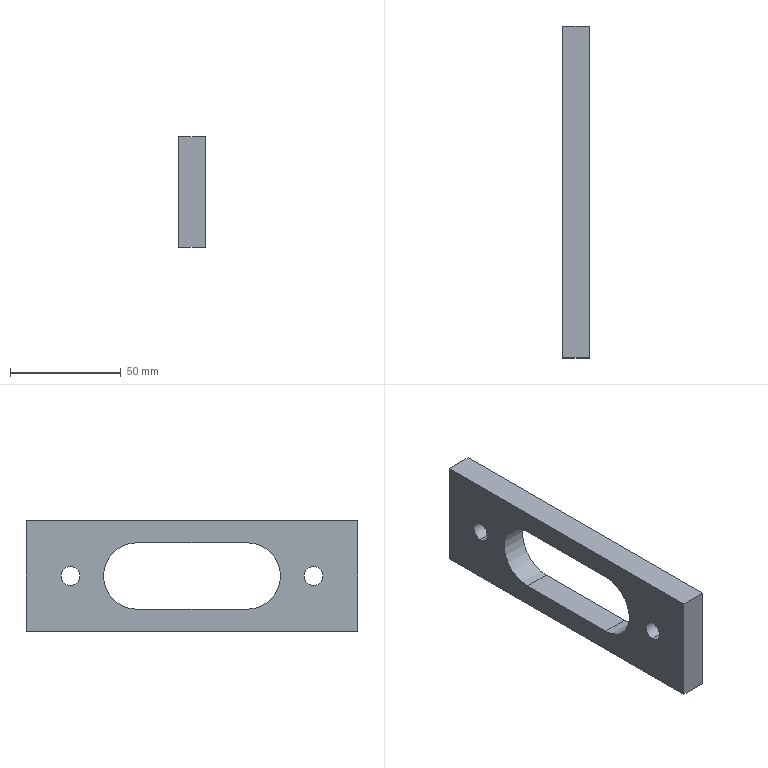Part | SolidWorks | features BaseBody 1 | 1 solid | 14 faces | box 12 x 150 x 50 mm | volume 62156 mm3 | plane 8 | cylinder 6 | commonest cylinder face diameters 8.5 x4 30 x2
STEP:
#1=CARTESIAN_POINT('',(-13.,224.,4.25));
#2=VERTEX_POINT('',#1);
#3=CARTESIAN_POINT('',(-13.,224.,-4.25));
#4=VERTEX_POINT('',#3);
#5=CARTESIAN_POINT('',(-13.,224.,0.));
#6=DIRECTION('',(1.,0.,0.));
#7=DIRECTION('',(0.,0.,-1.));
#8=AXIS2_PLACEMENT_3D('',#5,#6,#7);
#9=CIRCLE('',#8,4.25);
#10=EDGE_CURVE('',#2,#4,#9,.T.);
#11=ORIENTED_EDGE('',*,*,#10,.T.);
#12=CARTESIAN_POINT('',(-25.,224.,-4.25));
#13=VERTEX_POINT('',#12);
#14=CARTESIAN_POINT('',(-25.,224.,-4.25));
#15=DIRECTION('',(-1.,0.,0.));
#16=VECTOR('',#15,1000.);
#17=LINE('',#14,#16);
#18=EDGE_CURVE('',#4,#13,#17,.T.);
#19=ORIENTED_EDGE('',*,*,#18,.T.);
#20=CARTESIAN_POINT('',(-25.,224.,4.25));
#21=VERTEX_POINT('',#20);
#22=CARTESIAN_POINT('',(-25.,224.,0.));
#23=DIRECTION('',(1.,0.,0.));
#24=DIRECTION('',(0.,0.,1.));
#25=AXIS2_PLACEMENT_3D('',#22,#23,#24);
#26=CIRCLE('',#25,4.25);
#27=EDGE_CURVE('',#21,#13,#26,.T.);
#28=ORIENTED_EDGE('',*,*,#27,.F.);
#29=CARTESIAN_POINT('',(-25.,224.,4.25));
#30=DIRECTION('',(-1.,0.,0.));
#31=VECTOR('',#30,1000.);
#32=LINE('',#29,#31);
#33=EDGE_CURVE('',#2,#21,#32,.T.);
#34=ORIENTED_EDGE('',*,*,#33,.F.);
#35=EDGE_LOOP('',(#11,#19,#28,#34));
#36=FACE_OUTER_BOUND('',#35,.T.);
#37=CARTESIAN_POINT('',(-25.,224.,0.));
#38=DIRECTION('',(-1.,0.,0.));
#39=DIRECTION('',(0.,0.,1.));
#40=AXIS2_PLACEMENT_3D('',#37,#38,#39);
#41=CYLINDRICAL_SURFACE('',#40,4.25);
#42=ADVANCED_FACE('',(#36),#41,.F.);
#43=CARTESIAN_POINT('',(-13.,334.,4.25));
#44=VERTEX_POINT('',#43);
#45=CARTESIAN_POINT('',(-13.,334.,-4.25));
#46=VERTEX_POINT('',#45);
#47=CARTESIAN_POINT('',(-13.,334.,0.));
#48=DIRECTION('',(1.,0.,0.));
#49=DIRECTION('',(0.,0.,-1.));
#50=AXIS2_PLACEMENT_3D('',#47,#48,#49);
#51=CIRCLE('',#50,4.25);
#52=EDGE_CURVE('',#44,#46,#51,.T.);
#53=ORIENTED_EDGE('',*,*,#52,.T.);
#54=CARTESIAN_POINT('',(-25.,334.,-4.25));
#55=VERTEX_POINT('',#54);
#56=CARTESIAN_POINT('',(-25.,334.,-4.25));
#57=DIRECTION('',(-1.,0.,0.));
#58=VECTOR('',#57,1000.);
#59=LINE('',#56,#58);
#60=EDGE_CURVE('',#46,#55,#59,.T.);
#61=ORIENTED_EDGE('',*,*,#60,.T.);
#62=CARTESIAN_POINT('',(-25.,334.,4.25));
#63=VERTEX_POINT('',#62);
#64=CARTESIAN_POINT('',(-25.,334.,0.));
#65=DIRECTION('',(1.,0.,0.));
#66=DIRECTION('',(0.,0.,1.));
#67=AXIS2_PLACEMENT_3D('',#64,#65,#66);
#68=CIRCLE('',#67,4.25);
#69=EDGE_CURVE('',#63,#55,#68,.T.);
#70=ORIENTED_EDGE('',*,*,#69,.F.);
#71=CARTESIAN_POINT('',(-25.,334.,4.25));
#72=DIRECTION('',(-1.,0.,0.));
#73=VECTOR('',#72,1000.);
#74=LINE('',#71,#73);
#75=EDGE_CURVE('',#44,#63,#74,.T.);
#76=ORIENTED_EDGE('',*,*,#75,.F.);
#77=EDGE_LOOP('',(#53,#61,#70,#76));
#78=FACE_OUTER_BOUND('',#77,.T.);
#79=CARTESIAN_POINT('',(-25.,334.,0.));
#80=DIRECTION('',(-1.,0.,0.));
#81=DIRECTION('',(0.,0.,1.));
#82=AXIS2_PLACEMENT_3D('',#79,#80,#81);
#83=CYLINDRICAL_SURFACE('',#82,4.25);
#84=ADVANCED_FACE('',(#78),#83,.F.);
#85=CARTESIAN_POINT('',(-25.,254.,15.));
#86=VERTEX_POINT('',#85);
#87=CARTESIAN_POINT('',(-25.,304.,15.));
#88=VERTEX_POINT('',#87);
#89=CARTESIAN_POINT('',(-25.,533.,15.));
#90=DIRECTION('',(0.,1.,0.));
#91=VECTOR('',#90,1000.);
#92=LINE('',#89,#91);
#93=EDGE_CURVE('',#86,#88,#92,.T.);
#94=ORIENTED_EDGE('',*,*,#93,.T.);
#95=CARTESIAN_POINT('',(-13.,304.,15.));
#96=VERTEX_POINT('',#95);
#97=CARTESIAN_POINT('',(-13.,304.,15.));
#98=DIRECTION('',(1.,0.,0.));
#99=VECTOR('',#98,1000.);
#100=LINE('',#97,#99);
#101=EDGE_CURVE('',#88,#96,#100,.T.);
#102=ORIENTED_EDGE('',*,*,#101,.T.);
#103=CARTESIAN_POINT('',(-13.,254.,15.));
#104=VERTEX_POINT('',#103);
#105=CARTESIAN_POINT('',(-13.,294.,15.));
#106=DIRECTION('',(0.,-1.,0.));
#107=VECTOR('',#106,1000.);
#108=LINE('',#105,#107);
#109=EDGE_CURVE('',#96,#104,#108,.T.);
#110=ORIENTED_EDGE('',*,*,#109,.T.);
#111=CARTESIAN_POINT('',(-13.,254.,15.));
#112=DIRECTION('',(-1.,0.,0.));
#113=VECTOR('',#112,1000.);
#114=LINE('',#111,#113);
#115=EDGE_CURVE('',#104,#86,#114,.T.);
#116=ORIENTED_EDGE('',*,*,#115,.T.);
#117=EDGE_LOOP('',(#94,#102,#110,#116));
#118=FACE_OUTER_BOUND('',#117,.T.);
#119=CARTESIAN_POINT('',(-13.,294.,15.));
#120=DIRECTION('',(0.,0.,1.));
#121=DIRECTION('',(0.,-1.,0.));
#122=AXIS2_PLACEMENT_3D('',#119,#120,#121);
#123=PLANE('',#122);
#124=ADVANCED_FACE('',(#118),#123,.F.);
#125=CARTESIAN_POINT('',(-25.,304.,-15.));
#126=VERTEX_POINT('',#125);
#127=CARTESIAN_POINT('',(-25.,254.,-15.));
#128=VERTEX_POINT('',#127);
#129=CARTESIAN_POINT('',(-25.,533.,-15.));
#130=DIRECTION('',(0.,-1.,0.));
#131=VECTOR('',#130,1000.);
#132=LINE('',#129,#131);
#133=EDGE_CURVE('',#126,#128,#132,.T.);
#134=ORIENTED_EDGE('',*,*,#133,.T.);
#135=CARTESIAN_POINT('',(-13.,254.,-15.));
#136=VERTEX_POINT('',#135);
#137=CARTESIAN_POINT('',(-13.,254.,-15.));
#138=DIRECTION('',(1.,0.,0.));
#139=VECTOR('',#138,1000.);
#140=LINE('',#137,#139);
#141=EDGE_CURVE('',#128,#136,#140,.T.);
#142=ORIENTED_EDGE('',*,*,#141,.T.);
#143=CARTESIAN_POINT('',(-13.,304.,-15.));
#144=VERTEX_POINT('',#143);
#145=CARTESIAN_POINT('',(-13.,533.,-15.));
#146=DIRECTION('',(0.,-1.,0.));
#147=VECTOR('',#146,1000.);
#148=LINE('',#145,#147);
#149=EDGE_CURVE('',#144,#136,#148,.T.);
#150=ORIENTED_EDGE('',*,*,#149,.F.);
#151=CARTESIAN_POINT('',(-13.,304.,-15.));
#152=DIRECTION('',(-1.,0.,0.));
#153=VECTOR('',#152,1000.);
#154=LINE('',#151,#153);
#155=EDGE_CURVE('',#144,#126,#154,.T.);
#156=ORIENTED_EDGE('',*,*,#155,.T.);
#157=EDGE_LOOP('',(#134,#142,#150,#156));
#158=FACE_OUTER_BOUND('',#157,.T.);
#159=CARTESIAN_POINT('',(-13.,294.,-15.));
#160=DIRECTION('',(0.,0.,-1.));
#161=DIRECTION('',(-1.,0.,0.));
#162=AXIS2_PLACEMENT_3D('',#159,#160,#161);
#163=PLANE('',#162);
#164=ADVANCED_FACE('',(#158),#163,.F.);
#165=CARTESIAN_POINT('',(-25.,304.,0.));
#166=DIRECTION('',(-1.,0.,0.));
#167=DIRECTION('',(0.,0.,1.));
#168=AXIS2_PLACEMENT_3D('',#165,#166,#167);
#169=CIRCLE('',#168,15.);
#170=EDGE_CURVE('',#88,#126,#169,.T.);
#171=ORIENTED_EDGE('',*,*,#170,.T.);
#172=ORIENTED_EDGE('',*,*,#155,.F.);
#173=CARTESIAN_POINT('',(-13.,304.,0.));
#174=DIRECTION('',(1.,0.,0.));
#175=DIRECTION('',(0.,0.,1.));
#176=AXIS2_PLACEMENT_3D('',#173,#174,#175);
#177=CIRCLE('',#176,15.);
#178=EDGE_CURVE('',#144,#96,#177,.T.);
#179=ORIENTED_EDGE('',*,*,#178,.T.);
#180=ORIENTED_EDGE('',*,*,#101,.F.);
#181=EDGE_LOOP('',(#171,#172,#179,#180));
#182=FACE_OUTER_BOUND('',#181,.T.);
#183=CARTESIAN_POINT('',(-13.,304.,0.));
#184=DIRECTION('',(1.,0.,0.));
#185=DIRECTION('',(0.,0.,-1.));
#186=AXIS2_PLACEMENT_3D('',#183,#184,#185);
#187=CYLINDRICAL_SURFACE('',#186,15.);
#188=ADVANCED_FACE('',(#182),#187,.F.);
#189=CARTESIAN_POINT('',(-25.,254.,0.));
#190=DIRECTION('',(-1.,0.,0.));
#191=DIRECTION('',(0.,0.,1.));
#192=AXIS2_PLACEMENT_3D('',#189,#190,#191);
#193=CIRCLE('',#192,15.);
#194=EDGE_CURVE('',#128,#86,#193,.T.);
#195=ORIENTED_EDGE('',*,*,#194,.T.);
#196=ORIENTED_EDGE('',*,*,#115,.F.);
#197=CARTESIAN_POINT('',(-13.,254.,0.));
#198=DIRECTION('',(1.,0.,0.));
#199=DIRECTION('',(0.,0.,1.));
#200=AXIS2_PLACEMENT_3D('',#197,#198,#199);
#201=CIRCLE('',#200,15.);
#202=EDGE_CURVE('',#104,#136,#201,.T.);
#203=ORIENTED_EDGE('',*,*,#202,.T.);
#204=ORIENTED_EDGE('',*,*,#141,.F.);
#205=EDGE_LOOP('',(#195,#196,#203,#204));
#206=FACE_OUTER_BOUND('',#205,.T.);
#207=CARTESIAN_POINT('',(-13.,254.,0.));
#208=DIRECTION('',(1.,0.,0.));
#209=DIRECTION('',(0.,0.,-1.));
#210=AXIS2_PLACEMENT_3D('',#207,#208,#209);
#211=CYLINDRICAL_SURFACE('',#210,15.);
#212=ADVANCED_FACE('',(#206),#211,.F.);
#213=ORIENTED_EDGE('',*,*,#27,.T.);
#214=CARTESIAN_POINT('',(-25.,224.,0.));
#215=DIRECTION('',(1.,0.,0.));
#216=DIRECTION('',(0.,0.,1.));
#217=AXIS2_PLACEMENT_3D('',#214,#215,#216);
#218=CIRCLE('',#217,4.25);
#219=EDGE_CURVE('',#13,#21,#218,.T.);
#220=ORIENTED_EDGE('',*,*,#219,.T.);
#221=EDGE_LOOP('',(#213,#220));
#222=FACE_BOUND('',#221,.T.);
#223=ORIENTED_EDGE('',*,*,#69,.T.);
#224=CARTESIAN_POINT('',(-25.,334.,0.));
#225=DIRECTION('',(1.,0.,0.));
#226=DIRECTION('',(0.,0.,1.));
#227=AXIS2_PLACEMENT_3D('',#224,#225,#226);
#228=CIRCLE('',#227,4.25);
#229=EDGE_CURVE('',#55,#63,#228,.T.);
#230=ORIENTED_EDGE('',*,*,#229,.T.);
#231=EDGE_LOOP('',(#223,#230));
#232=FACE_BOUND('',#231,.T.);
#233=ORIENTED_EDGE('',*,*,#194,.F.);
#234=ORIENTED_EDGE('',*,*,#133,.F.);
#235=ORIENTED_EDGE('',*,*,#170,.F.);
#236=ORIENTED_EDGE('',*,*,#93,.F.);
#237=EDGE_LOOP('',(#233,#234,#235,#236));
#238=FACE_BOUND('',#237,.T.);
#239=CARTESIAN_POINT('',(-25.,204.,-25.));
#240=VERTEX_POINT('',#239);
#241=CARTESIAN_POINT('',(-25.,354.,-25.));
#242=VERTEX_POINT('',#241);
#243=CARTESIAN_POINT('',(-25.,204.,-25.));
#244=DIRECTION('',(0.,1.,0.));
#245=VECTOR('',#244,1000.);
#246=LINE('',#243,#245);
#247=EDGE_CURVE('',#240,#242,#246,.T.);
#248=ORIENTED_EDGE('',*,*,#247,.F.);
#249=CARTESIAN_POINT('',(-25.,204.,25.));
#250=VERTEX_POINT('',#249);
#251=CARTESIAN_POINT('',(-25.,204.,-25.));
#252=DIRECTION('',(0.,0.,-1.));
#253=VECTOR('',#252,1000.);
#254=LINE('',#251,#253);
#255=EDGE_CURVE('',#250,#240,#254,.T.);
#256=ORIENTED_EDGE('',*,*,#255,.F.);
#257=CARTESIAN_POINT('',(-25.,354.,25.));
#258=VERTEX_POINT('',#257);
#259=CARTESIAN_POINT('',(-25.,204.,25.));
#260=DIRECTION('',(0.,-1.,0.));
#261=VECTOR('',#260,1000.);
#262=LINE('',#259,#261);
#263=EDGE_CURVE('',#258,#250,#262,.T.);
#264=ORIENTED_EDGE('',*,*,#263,.F.);
#265=CARTESIAN_POINT('',(-25.,354.,-25.));
#266=DIRECTION('',(0.,0.,1.));
#267=VECTOR('',#266,1000.);
#268=LINE('',#265,#267);
#269=EDGE_CURVE('',#242,#258,#268,.T.);
#270=ORIENTED_EDGE('',*,*,#269,.F.);
#271=EDGE_LOOP('',(#248,#256,#264,#270));
#272=FACE_OUTER_BOUND('',#271,.T.);
#273=CARTESIAN_POINT('',(-25.,533.,0.));
#274=DIRECTION('',(-1.,0.,0.));
#275=DIRECTION('',(0.,1.,0.));
#276=AXIS2_PLACEMENT_3D('',#273,#274,#275);
#277=PLANE('',#276);
#278=ADVANCED_FACE('',(#222,#232,#238,#272),#277,.T.);
#279=ORIENTED_EDGE('',*,*,#269,.T.);
#280=CARTESIAN_POINT('',(-13.,354.,25.));
#281=VERTEX_POINT('',#280);
#282=CARTESIAN_POINT('',(-25.,354.,25.));
#283=DIRECTION('',(1.,0.,0.));
#284=VECTOR('',#283,1000.);
#285=LINE('',#282,#284);
#286=EDGE_CURVE('',#258,#281,#285,.T.);
#287=ORIENTED_EDGE('',*,*,#286,.T.);
#288=CARTESIAN_POINT('',(-13.,354.,-25.));
#289=VERTEX_POINT('',#288);
#290=CARTESIAN_POINT('',(-13.,354.,0.));
#291=DIRECTION('',(0.,0.,1.));
#292=VECTOR('',#291,1000.);
#293=LINE('',#290,#292);
#294=EDGE_CURVE('',#289,#281,#293,.T.);
#295=ORIENTED_EDGE('',*,*,#294,.F.);
#296=CARTESIAN_POINT('',(-25.,354.,-25.));
#297=DIRECTION('',(1.,0.,0.));
#298=VECTOR('',#297,1000.);
#299=LINE('',#296,#298);
#300=EDGE_CURVE('',#242,#289,#299,.T.);
#301=ORIENTED_EDGE('',*,*,#300,.F.);
#302=EDGE_LOOP('',(#279,#287,#295,#301));
#303=FACE_OUTER_BOUND('',#302,.T.);
#304=CARTESIAN_POINT('',(-25.,354.,-25.));
#305=DIRECTION('',(0.,-1.,0.));
#306=DIRECTION('',(0.,0.,-1.));
#307=AXIS2_PLACEMENT_3D('',#304,#305,#306);
#308=PLANE('',#307);
#309=ADVANCED_FACE('',(#303),#308,.F.);
#310=CARTESIAN_POINT('',(-13.,204.,-25.));
#311=VERTEX_POINT('',#310);
#312=CARTESIAN_POINT('',(-25.,204.,-25.));
#313=DIRECTION('',(1.,0.,0.));
#314=VECTOR('',#313,1000.);
#315=LINE('',#312,#314);
#316=EDGE_CURVE('',#240,#311,#315,.T.);
#317=ORIENTED_EDGE('',*,*,#316,.F.);
#318=ORIENTED_EDGE('',*,*,#247,.T.);
#319=ORIENTED_EDGE('',*,*,#300,.T.);
#320=CARTESIAN_POINT('',(-13.,533.,-25.));
#321=DIRECTION('',(0.,1.,0.));
#322=VECTOR('',#321,1000.);
#323=LINE('',#320,#322);
#324=EDGE_CURVE('',#311,#289,#323,.T.);
#325=ORIENTED_EDGE('',*,*,#324,.F.);
#326=EDGE_LOOP('',(#317,#318,#319,#325));
#327=FACE_OUTER_BOUND('',#326,.T.);
#328=CARTESIAN_POINT('',(-25.,204.,-25.));
#329=DIRECTION('',(0.,0.,1.));
#330=DIRECTION('',(0.,-1.,0.));
#331=AXIS2_PLACEMENT_3D('',#328,#329,#330);
#332=PLANE('',#331);
#333=ADVANCED_FACE('',(#327),#332,.F.);
#334=CARTESIAN_POINT('',(-13.,204.,25.));
#335=VERTEX_POINT('',#334);
#336=CARTESIAN_POINT('',(-25.,204.,25.));
#337=DIRECTION('',(1.,0.,0.));
#338=VECTOR('',#337,1000.);
#339=LINE('',#336,#338);
#340=EDGE_CURVE('',#250,#335,#339,.T.);
#341=ORIENTED_EDGE('',*,*,#340,.F.);
#342=ORIENTED_EDGE('',*,*,#255,.T.);
#343=ORIENTED_EDGE('',*,*,#316,.T.);
#344=CARTESIAN_POINT('',(-13.,204.,0.));
#345=DIRECTION('',(0.,0.,-1.));
#346=VECTOR('',#345,1000.);
#347=LINE('',#344,#346);
#348=EDGE_CURVE('',#335,#311,#347,.T.);
#349=ORIENTED_EDGE('',*,*,#348,.F.);
#350=EDGE_LOOP('',(#341,#342,#343,#349));
#351=FACE_OUTER_BOUND('',#350,.T.);
#352=CARTESIAN_POINT('',(-25.,204.,-25.));
#353=DIRECTION('',(0.,1.,0.));
#354=DIRECTION('',(0.,0.,-1.));
#355=AXIS2_PLACEMENT_3D('',#352,#353,#354);
#356=PLANE('',#355);
#357=ADVANCED_FACE('',(#351),#356,.F.);
#358=ORIENTED_EDGE('',*,*,#286,.F.);
#359=ORIENTED_EDGE('',*,*,#263,.T.);
#360=ORIENTED_EDGE('',*,*,#340,.T.);
#361=CARTESIAN_POINT('',(-13.,533.,25.));
#362=DIRECTION('',(0.,-1.,0.));
#363=VECTOR('',#362,1000.);
#364=LINE('',#361,#363);
#365=EDGE_CURVE('',#281,#335,#364,.T.);
#366=ORIENTED_EDGE('',*,*,#365,.F.);
#367=EDGE_LOOP('',(#358,#359,#360,#366));
#368=FACE_OUTER_BOUND('',#367,.T.);
#369=CARTESIAN_POINT('',(-25.,204.,25.));
#370=DIRECTION('',(0.,0.,-1.));
#371=DIRECTION('',(0.,-1.,0.));
#372=AXIS2_PLACEMENT_3D('',#369,#370,#371);
#373=PLANE('',#372);
#374=ADVANCED_FACE('',(#368),#373,.F.);
#375=ORIENTED_EDGE('',*,*,#178,.F.);
#376=ORIENTED_EDGE('',*,*,#149,.T.);
#377=ORIENTED_EDGE('',*,*,#202,.F.);
#378=ORIENTED_EDGE('',*,*,#109,.F.);
#379=EDGE_LOOP('',(#375,#376,#377,#378));
#380=FACE_BOUND('',#379,.T.);
#381=ORIENTED_EDGE('',*,*,#52,.F.);
#382=CARTESIAN_POINT('',(-13.,334.,0.));
#383=DIRECTION('',(1.,0.,0.));
#384=DIRECTION('',(0.,0.,-1.));
#385=AXIS2_PLACEMENT_3D('',#382,#383,#384);
#386=CIRCLE('',#385,4.25);
#387=EDGE_CURVE('',#46,#44,#386,.T.);
#388=ORIENTED_EDGE('',*,*,#387,.F.);
#389=EDGE_LOOP('',(#381,#388));
#390=FACE_BOUND('',#389,.T.);
#391=ORIENTED_EDGE('',*,*,#10,.F.);
#392=CARTESIAN_POINT('',(-13.,224.,0.));
#393=DIRECTION('',(1.,0.,0.));
#394=DIRECTION('',(0.,0.,-1.));
#395=AXIS2_PLACEMENT_3D('',#392,#393,#394);
#396=CIRCLE('',#395,4.25);
#397=EDGE_CURVE('',#4,#2,#396,.T.);
#398=ORIENTED_EDGE('',*,*,#397,.F.);
#399=EDGE_LOOP('',(#391,#398));
#400=FACE_BOUND('',#399,.T.);
#401=ORIENTED_EDGE('',*,*,#324,.T.);
#402=ORIENTED_EDGE('',*,*,#294,.T.);
#403=ORIENTED_EDGE('',*,*,#365,.T.);
#404=ORIENTED_EDGE('',*,*,#348,.T.);
#405=EDGE_LOOP('',(#401,#402,#403,#404));
#406=FACE_OUTER_BOUND('',#405,.T.);
#407=CARTESIAN_POINT('',(-13.,533.,0.));
#408=DIRECTION('',(-1.,0.,0.));
#409=DIRECTION('',(0.,1.,0.));
#410=AXIS2_PLACEMENT_3D('',#407,#408,#409);
#411=PLANE('',#410);
#412=ADVANCED_FACE('',(#380,#390,#400,#406),#411,.F.);
#413=ORIENTED_EDGE('',*,*,#60,.F.);
#414=ORIENTED_EDGE('',*,*,#387,.T.);
#415=ORIENTED_EDGE('',*,*,#75,.T.);
#416=ORIENTED_EDGE('',*,*,#229,.F.);
#417=EDGE_LOOP('',(#413,#414,#415,#416));
#418=FACE_OUTER_BOUND('',#417,.T.);
#419=CARTESIAN_POINT('',(-25.,334.,0.));
#420=DIRECTION('',(-1.,0.,0.));
#421=DIRECTION('',(0.,0.,1.));
#422=AXIS2_PLACEMENT_3D('',#419,#420,#421);
#423=CYLINDRICAL_SURFACE('',#422,4.25);
#424=ADVANCED_FACE('',(#418),#423,.F.);
#425=ORIENTED_EDGE('',*,*,#18,.F.);
#426=ORIENTED_EDGE('',*,*,#397,.T.);
#427=ORIENTED_EDGE('',*,*,#33,.T.);
#428=ORIENTED_EDGE('',*,*,#219,.F.);
#429=EDGE_LOOP('',(#425,#426,#427,#428));
#430=FACE_OUTER_BOUND('',#429,.T.);
#431=CARTESIAN_POINT('',(-25.,224.,0.));
#432=DIRECTION('',(-1.,0.,0.));
#433=DIRECTION('',(0.,0.,1.));
#434=AXIS2_PLACEMENT_3D('',#431,#432,#433);
#435=CYLINDRICAL_SURFACE('',#434,4.25);
#436=ADVANCED_FACE('',(#430),#435,.F.);
#437=CLOSED_SHELL('',(#42,#84,#124,#164,#188,#212,#278,#309,#333,#357,#374,#412,#424,#436));
#438=MANIFOLD_SOLID_BREP('',#437);
#439=CARTESIAN_POINT('',(0.,0.,0.));
#440=DIRECTION('',(0.,0.,1.));
#441=DIRECTION('',(1.,0.,0.));
#442=AXIS2_PLACEMENT_3D('',#439,#440,#441);
#443=(LENGTH_UNIT()NAMED_UNIT(*)SI_UNIT(.MILLI.,.METRE.));
#444=UNCERTAINTY_MEASURE_WITH_UNIT(LENGTH_MEASURE(0.00001),#443,'','');
#445=(NAMED_UNIT(*)PLANE_ANGLE_UNIT()SI_UNIT($,.RADIAN.));
#446=(NAMED_UNIT(*)SI_UNIT($,.STERADIAN.)SOLID_ANGLE_UNIT());
#447=(GEOMETRIC_REPRESENTATION_CONTEXT(3)GLOBAL_UNCERTAINTY_ASSIGNED_CONTEXT((#444))GLOBAL_UNIT_ASSIGNED_CONTEXT((#443,#445,#446))REPRESENTATION_CONTEXT('',''));
#448=ADVANCED_BREP_SHAPE_REPRESENTATION('',(#438,#442),#447);